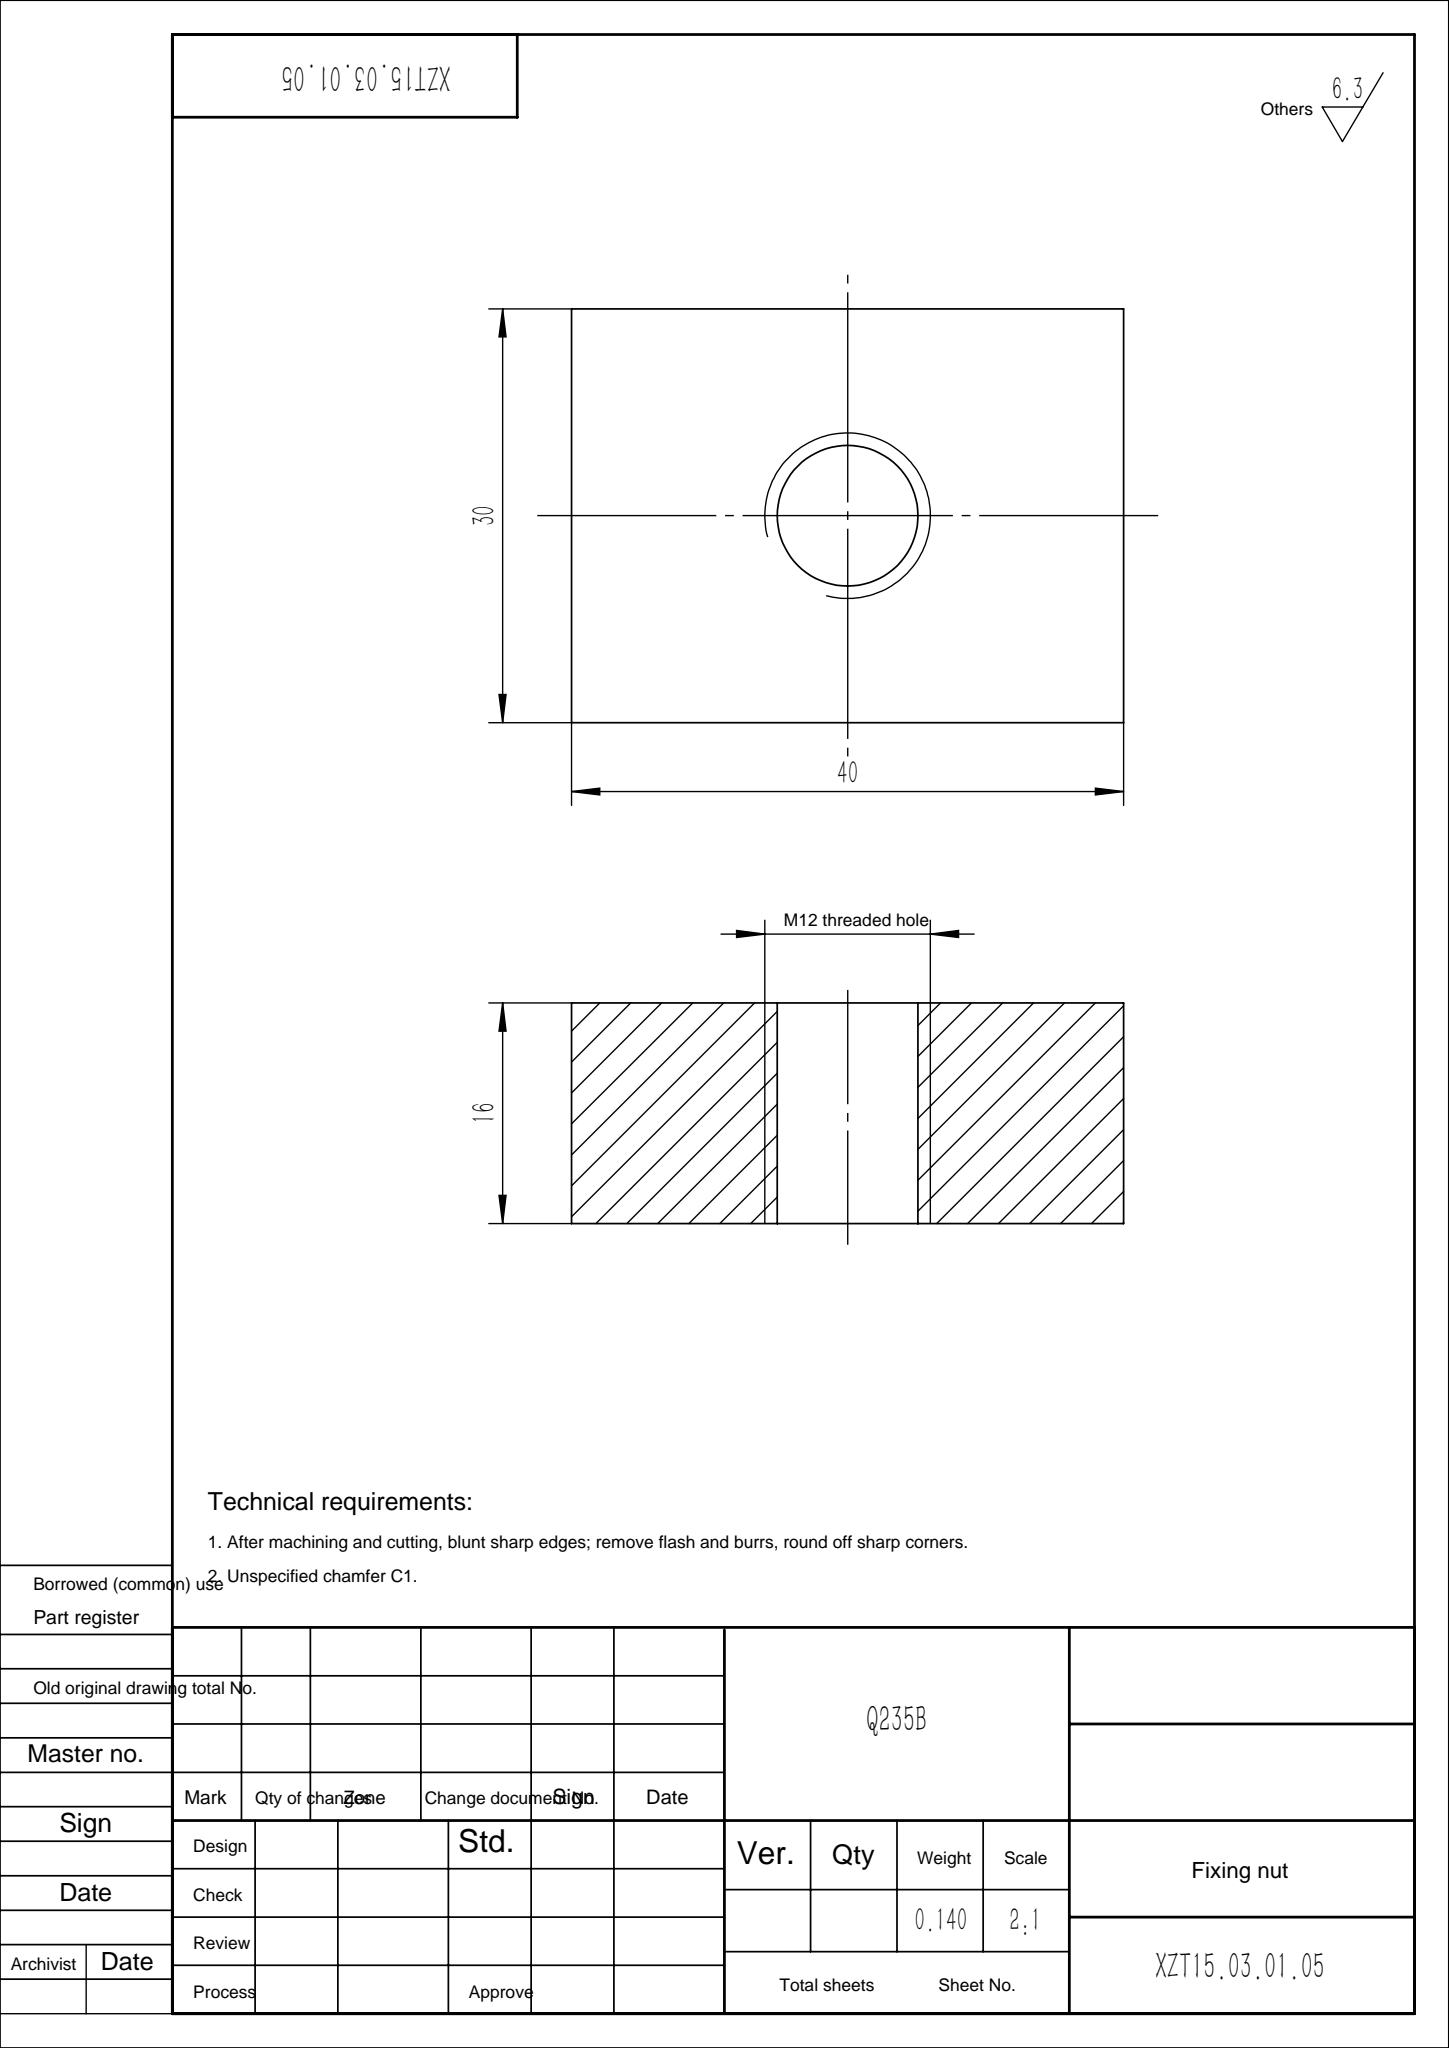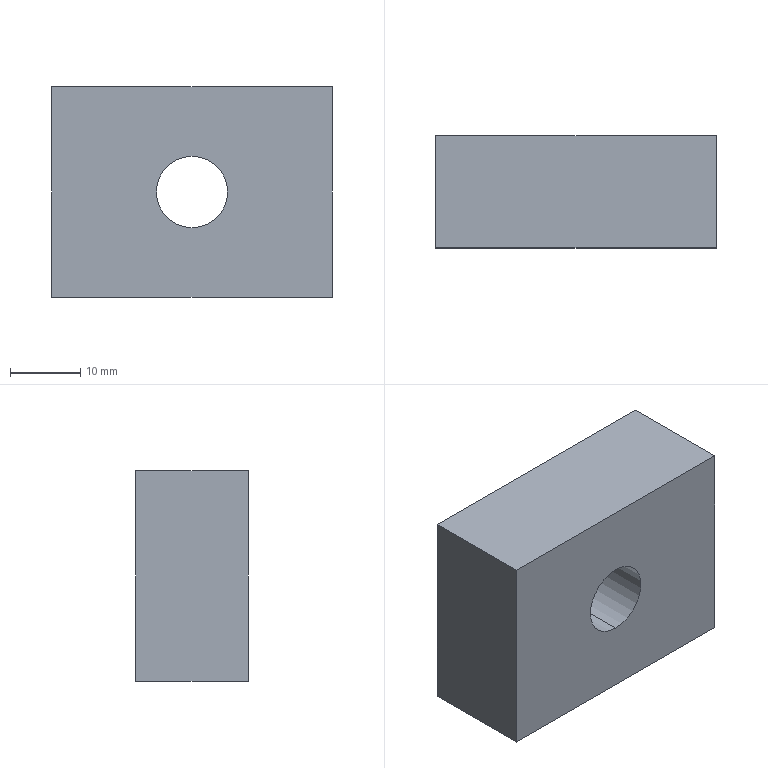Part | SolidWorks | features Extrusion 1, HoleWzd 1 | 1 solid | 8 faces | box 40 x 16 x 30 mm | volume 17893 mm3 | plane 6 | cylinder 2 | commonest cylinder face diameters 10.2 x2
STEP:
#1=CARTESIAN_POINT('',(0.,0.,-5.1));
#2=VERTEX_POINT('',#1);
#3=CARTESIAN_POINT('',(0.,0.,5.1));
#4=VERTEX_POINT('',#3);
#5=CARTESIAN_POINT('',(0.,0.,0.));
#6=DIRECTION('',(0.,1.,0.));
#7=DIRECTION('',(0.,0.,1.));
#8=AXIS2_PLACEMENT_3D('',#5,#6,#7);
#9=CIRCLE('',#8,5.1);
#10=EDGE_CURVE('',#2,#4,#9,.T.);
#11=ORIENTED_EDGE('',*,*,#10,.F.);
#12=CARTESIAN_POINT('',(0.,16.,-5.1));
#13=VERTEX_POINT('',#12);
#14=CARTESIAN_POINT('',(0.,16.,-5.1));
#15=DIRECTION('',(0.,1.,0.));
#16=VECTOR('',#15,1000.);
#17=LINE('',#14,#16);
#18=EDGE_CURVE('',#2,#13,#17,.T.);
#19=ORIENTED_EDGE('',*,*,#18,.T.);
#20=CARTESIAN_POINT('',(0.,16.,5.1));
#21=VERTEX_POINT('',#20);
#22=CARTESIAN_POINT('',(0.,16.,0.));
#23=DIRECTION('',(0.,1.,0.));
#24=DIRECTION('',(0.,0.,1.));
#25=AXIS2_PLACEMENT_3D('',#22,#23,#24);
#26=CIRCLE('',#25,5.1);
#27=EDGE_CURVE('',#13,#21,#26,.T.);
#28=ORIENTED_EDGE('',*,*,#27,.T.);
#29=CARTESIAN_POINT('',(0.,16.,5.1));
#30=DIRECTION('',(0.,1.,0.));
#31=VECTOR('',#30,1000.);
#32=LINE('',#29,#31);
#33=EDGE_CURVE('',#4,#21,#32,.T.);
#34=ORIENTED_EDGE('',*,*,#33,.F.);
#35=EDGE_LOOP('',(#11,#19,#28,#34));
#36=FACE_OUTER_BOUND('',#35,.T.);
#37=CARTESIAN_POINT('',(0.,16.,0.));
#38=DIRECTION('',(0.,1.,0.));
#39=DIRECTION('',(0.,0.,1.));
#40=AXIS2_PLACEMENT_3D('',#37,#38,#39);
#41=CYLINDRICAL_SURFACE('',#40,5.1);
#42=ADVANCED_FACE('',(#36),#41,.F.);
#43=CARTESIAN_POINT('',(-20.,0.,-15.));
#44=VERTEX_POINT('',#43);
#45=CARTESIAN_POINT('',(-20.,0.,15.));
#46=VERTEX_POINT('',#45);
#47=CARTESIAN_POINT('',(-20.,0.,15.));
#48=DIRECTION('',(0.,0.,1.));
#49=VECTOR('',#48,1000.);
#50=LINE('',#47,#49);
#51=EDGE_CURVE('',#44,#46,#50,.T.);
#52=ORIENTED_EDGE('',*,*,#51,.T.);
#53=CARTESIAN_POINT('',(-20.,16.,15.));
#54=VERTEX_POINT('',#53);
#55=CARTESIAN_POINT('',(-20.,16.,15.));
#56=DIRECTION('',(0.,-1.,0.));
#57=VECTOR('',#56,1000.);
#58=LINE('',#55,#57);
#59=EDGE_CURVE('',#54,#46,#58,.T.);
#60=ORIENTED_EDGE('',*,*,#59,.F.);
#61=CARTESIAN_POINT('',(-20.,16.,-15.));
#62=VERTEX_POINT('',#61);
#63=CARTESIAN_POINT('',(-20.,16.,15.));
#64=DIRECTION('',(0.,0.,1.));
#65=VECTOR('',#64,1000.);
#66=LINE('',#63,#65);
#67=EDGE_CURVE('',#62,#54,#66,.T.);
#68=ORIENTED_EDGE('',*,*,#67,.F.);
#69=CARTESIAN_POINT('',(-20.,16.,-15.));
#70=DIRECTION('',(0.,-1.,0.));
#71=VECTOR('',#70,1000.);
#72=LINE('',#69,#71);
#73=EDGE_CURVE('',#62,#44,#72,.T.);
#74=ORIENTED_EDGE('',*,*,#73,.T.);
#75=EDGE_LOOP('',(#52,#60,#68,#74));
#76=FACE_OUTER_BOUND('',#75,.T.);
#77=CARTESIAN_POINT('',(-20.,16.,15.));
#78=DIRECTION('',(1.,0.,0.));
#79=DIRECTION('',(0.,0.,-1.));
#80=AXIS2_PLACEMENT_3D('',#77,#78,#79);
#81=PLANE('',#80);
#82=ADVANCED_FACE('',(#76),#81,.F.);
#83=CARTESIAN_POINT('',(20.,0.,15.));
#84=VERTEX_POINT('',#83);
#85=CARTESIAN_POINT('',(20.,0.,15.));
#86=DIRECTION('',(1.,0.,0.));
#87=VECTOR('',#86,1000.);
#88=LINE('',#85,#87);
#89=EDGE_CURVE('',#46,#84,#88,.T.);
#90=ORIENTED_EDGE('',*,*,#89,.T.);
#91=CARTESIAN_POINT('',(20.,16.,15.));
#92=VERTEX_POINT('',#91);
#93=CARTESIAN_POINT('',(20.,16.,15.));
#94=DIRECTION('',(0.,-1.,0.));
#95=VECTOR('',#94,1000.);
#96=LINE('',#93,#95);
#97=EDGE_CURVE('',#92,#84,#96,.T.);
#98=ORIENTED_EDGE('',*,*,#97,.F.);
#99=CARTESIAN_POINT('',(20.,16.,15.));
#100=DIRECTION('',(1.,0.,0.));
#101=VECTOR('',#100,1000.);
#102=LINE('',#99,#101);
#103=EDGE_CURVE('',#54,#92,#102,.T.);
#104=ORIENTED_EDGE('',*,*,#103,.F.);
#105=ORIENTED_EDGE('',*,*,#59,.T.);
#106=EDGE_LOOP('',(#90,#98,#104,#105));
#107=FACE_OUTER_BOUND('',#106,.T.);
#108=CARTESIAN_POINT('',(20.,16.,15.));
#109=DIRECTION('',(0.,0.,-1.));
#110=DIRECTION('',(-1.,0.,0.));
#111=AXIS2_PLACEMENT_3D('',#108,#109,#110);
#112=PLANE('',#111);
#113=ADVANCED_FACE('',(#107),#112,.F.);
#114=CARTESIAN_POINT('',(20.,0.,-15.));
#115=VERTEX_POINT('',#114);
#116=CARTESIAN_POINT('',(20.,0.,15.));
#117=DIRECTION('',(0.,0.,-1.));
#118=VECTOR('',#117,1000.);
#119=LINE('',#116,#118);
#120=EDGE_CURVE('',#84,#115,#119,.T.);
#121=ORIENTED_EDGE('',*,*,#120,.T.);
#122=CARTESIAN_POINT('',(20.,16.,-15.));
#123=VERTEX_POINT('',#122);
#124=CARTESIAN_POINT('',(20.,16.,-15.));
#125=DIRECTION('',(0.,-1.,0.));
#126=VECTOR('',#125,1000.);
#127=LINE('',#124,#126);
#128=EDGE_CURVE('',#123,#115,#127,.T.);
#129=ORIENTED_EDGE('',*,*,#128,.F.);
#130=CARTESIAN_POINT('',(20.,16.,15.));
#131=DIRECTION('',(0.,0.,-1.));
#132=VECTOR('',#131,1000.);
#133=LINE('',#130,#132);
#134=EDGE_CURVE('',#92,#123,#133,.T.);
#135=ORIENTED_EDGE('',*,*,#134,.F.);
#136=ORIENTED_EDGE('',*,*,#97,.T.);
#137=EDGE_LOOP('',(#121,#129,#135,#136));
#138=FACE_OUTER_BOUND('',#137,.T.);
#139=CARTESIAN_POINT('',(20.,16.,15.));
#140=DIRECTION('',(-1.,0.,0.));
#141=DIRECTION('',(0.,0.,1.));
#142=AXIS2_PLACEMENT_3D('',#139,#140,#141);
#143=PLANE('',#142);
#144=ADVANCED_FACE('',(#138),#143,.F.);
#145=CARTESIAN_POINT('',(20.,0.,-15.));
#146=DIRECTION('',(-1.,0.,0.));
#147=VECTOR('',#146,1000.);
#148=LINE('',#145,#147);
#149=EDGE_CURVE('',#115,#44,#148,.T.);
#150=ORIENTED_EDGE('',*,*,#149,.T.);
#151=ORIENTED_EDGE('',*,*,#73,.F.);
#152=CARTESIAN_POINT('',(20.,16.,-15.));
#153=DIRECTION('',(-1.,0.,0.));
#154=VECTOR('',#153,1000.);
#155=LINE('',#152,#154);
#156=EDGE_CURVE('',#123,#62,#155,.T.);
#157=ORIENTED_EDGE('',*,*,#156,.F.);
#158=ORIENTED_EDGE('',*,*,#128,.T.);
#159=EDGE_LOOP('',(#150,#151,#157,#158));
#160=FACE_OUTER_BOUND('',#159,.T.);
#161=CARTESIAN_POINT('',(20.,16.,-15.));
#162=DIRECTION('',(0.,0.,1.));
#163=DIRECTION('',(1.,0.,0.));
#164=AXIS2_PLACEMENT_3D('',#161,#162,#163);
#165=PLANE('',#164);
#166=ADVANCED_FACE('',(#160),#165,.F.);
#167=CARTESIAN_POINT('',(0.,16.,0.));
#168=DIRECTION('',(0.,1.,0.));
#169=DIRECTION('',(0.,0.,1.));
#170=AXIS2_PLACEMENT_3D('',#167,#168,#169);
#171=CIRCLE('',#170,5.1);
#172=EDGE_CURVE('',#21,#13,#171,.T.);
#173=ORIENTED_EDGE('',*,*,#172,.F.);
#174=ORIENTED_EDGE('',*,*,#27,.F.);
#175=EDGE_LOOP('',(#173,#174));
#176=FACE_BOUND('',#175,.T.);
#177=ORIENTED_EDGE('',*,*,#67,.T.);
#178=ORIENTED_EDGE('',*,*,#103,.T.);
#179=ORIENTED_EDGE('',*,*,#134,.T.);
#180=ORIENTED_EDGE('',*,*,#156,.T.);
#181=EDGE_LOOP('',(#177,#178,#179,#180));
#182=FACE_OUTER_BOUND('',#181,.T.);
#183=CARTESIAN_POINT('',(0.,16.,0.));
#184=DIRECTION('',(0.,1.,0.));
#185=DIRECTION('',(0.,0.,1.));
#186=AXIS2_PLACEMENT_3D('',#183,#184,#185);
#187=PLANE('',#186);
#188=ADVANCED_FACE('',(#176,#182),#187,.T.);
#189=CARTESIAN_POINT('',(0.,0.,0.));
#190=DIRECTION('',(0.,1.,0.));
#191=DIRECTION('',(0.,0.,1.));
#192=AXIS2_PLACEMENT_3D('',#189,#190,#191);
#193=CIRCLE('',#192,5.1);
#194=EDGE_CURVE('',#4,#2,#193,.T.);
#195=ORIENTED_EDGE('',*,*,#194,.T.);
#196=ORIENTED_EDGE('',*,*,#10,.T.);
#197=EDGE_LOOP('',(#195,#196));
#198=FACE_BOUND('',#197,.T.);
#199=ORIENTED_EDGE('',*,*,#51,.F.);
#200=ORIENTED_EDGE('',*,*,#149,.F.);
#201=ORIENTED_EDGE('',*,*,#120,.F.);
#202=ORIENTED_EDGE('',*,*,#89,.F.);
#203=EDGE_LOOP('',(#199,#200,#201,#202));
#204=FACE_OUTER_BOUND('',#203,.T.);
#205=CARTESIAN_POINT('',(0.,0.,0.));
#206=DIRECTION('',(0.,1.,0.));
#207=DIRECTION('',(0.,0.,1.));
#208=AXIS2_PLACEMENT_3D('',#205,#206,#207);
#209=PLANE('',#208);
#210=ADVANCED_FACE('',(#198,#204),#209,.F.);
#211=ORIENTED_EDGE('',*,*,#18,.F.);
#212=ORIENTED_EDGE('',*,*,#194,.F.);
#213=ORIENTED_EDGE('',*,*,#33,.T.);
#214=ORIENTED_EDGE('',*,*,#172,.T.);
#215=EDGE_LOOP('',(#211,#212,#213,#214));
#216=FACE_OUTER_BOUND('',#215,.T.);
#217=CARTESIAN_POINT('',(0.,16.,0.));
#218=DIRECTION('',(0.,1.,0.));
#219=DIRECTION('',(0.,0.,1.));
#220=AXIS2_PLACEMENT_3D('',#217,#218,#219);
#221=CYLINDRICAL_SURFACE('',#220,5.1);
#222=ADVANCED_FACE('',(#216),#221,.F.);
#223=CLOSED_SHELL('',(#42,#82,#113,#144,#166,#188,#210,#222));
#224=MANIFOLD_SOLID_BREP('',#223);
#225=CARTESIAN_POINT('',(0.,0.,0.));
#226=DIRECTION('',(0.,0.,1.));
#227=DIRECTION('',(1.,0.,0.));
#228=AXIS2_PLACEMENT_3D('',#225,#226,#227);
#229=(LENGTH_UNIT()NAMED_UNIT(*)SI_UNIT(.MILLI.,.METRE.));
#230=UNCERTAINTY_MEASURE_WITH_UNIT(LENGTH_MEASURE(0.00001),#229,'','');
#231=(NAMED_UNIT(*)PLANE_ANGLE_UNIT()SI_UNIT($,.RADIAN.));
#232=(NAMED_UNIT(*)SI_UNIT($,.STERADIAN.)SOLID_ANGLE_UNIT());
#233=(GEOMETRIC_REPRESENTATION_CONTEXT(3)GLOBAL_UNCERTAINTY_ASSIGNED_CONTEXT((#230))GLOBAL_UNIT_ASSIGNED_CONTEXT((#229,#231,#232))REPRESENTATION_CONTEXT('',''));
#234=ADVANCED_BREP_SHAPE_REPRESENTATION('',(#224,#228),#233);